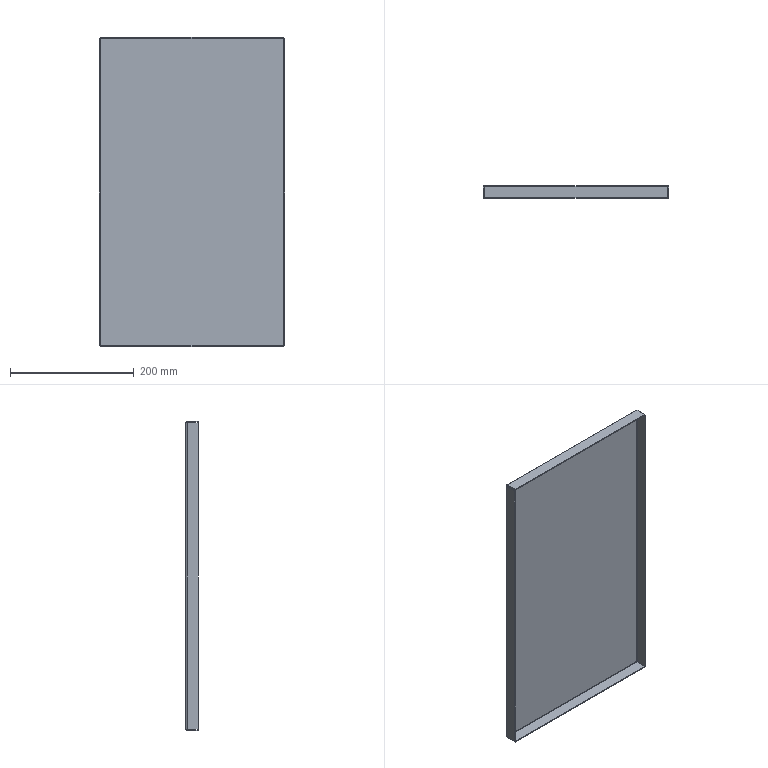Part | STEP file | PN_0072 base plate | 1 solid | 38 faces | box 300 x 20 x 500 mm | volume 267366 mm3 | plane 22 | spline 8 | cylinder 8 | commonest cylinder face diameters 1.473 x4 4.473 x4